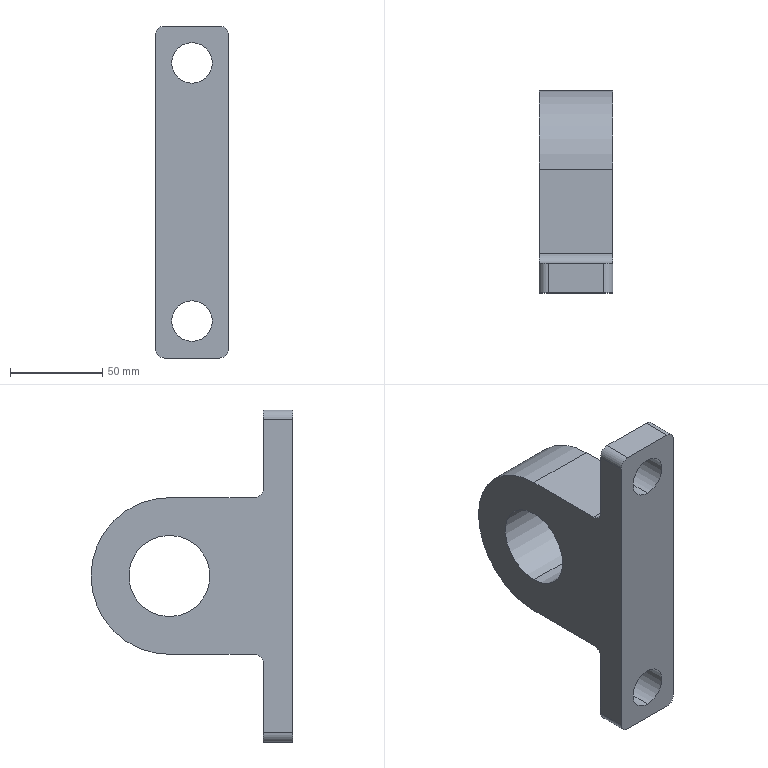Part | SolidWorks | features Extrusion 1, Fillet 1, ICE 1 | 1 solid | 22 faces | box 40 x 109.5 x 180 mm | volume 329190 mm3 | cylinder 13 | plane 9 | commonest cylinder face diameters 10 x6 22 x4 44 x2 85 x1
STEP:
#1=CARTESIAN_POINT('',(20.,67.,22.));
#2=VERTEX_POINT('',#1);
#3=CARTESIAN_POINT('',(20.,67.,-22.));
#4=VERTEX_POINT('',#3);
#5=CARTESIAN_POINT('',(20.,67.,0.));
#6=DIRECTION('',(1.,0.,0.));
#7=DIRECTION('',(0.,0.,-1.));
#8=AXIS2_PLACEMENT_3D('',#5,#6,#7);
#9=CIRCLE('',#8,22.);
#10=EDGE_CURVE('',#2,#4,#9,.T.);
#11=ORIENTED_EDGE('',*,*,#10,.T.);
#12=CARTESIAN_POINT('',(-20.,67.,-22.));
#13=VERTEX_POINT('',#12);
#14=CARTESIAN_POINT('',(20.,67.,-22.));
#15=DIRECTION('',(-1.,0.,0.));
#16=VECTOR('',#15,1000.);
#17=LINE('',#14,#16);
#18=EDGE_CURVE('',#4,#13,#17,.T.);
#19=ORIENTED_EDGE('',*,*,#18,.T.);
#20=CARTESIAN_POINT('',(-20.,67.,22.));
#21=VERTEX_POINT('',#20);
#22=CARTESIAN_POINT('',(-20.,67.,0.));
#23=DIRECTION('',(1.,0.,0.));
#24=DIRECTION('',(0.,0.,-1.));
#25=AXIS2_PLACEMENT_3D('',#22,#23,#24);
#26=CIRCLE('',#25,22.);
#27=EDGE_CURVE('',#21,#13,#26,.T.);
#28=ORIENTED_EDGE('',*,*,#27,.F.);
#29=CARTESIAN_POINT('',(20.,67.,22.));
#30=DIRECTION('',(-1.,0.,0.));
#31=VECTOR('',#30,1000.);
#32=LINE('',#29,#31);
#33=EDGE_CURVE('',#2,#21,#32,.T.);
#34=ORIENTED_EDGE('',*,*,#33,.F.);
#35=EDGE_LOOP('',(#11,#19,#28,#34));
#36=FACE_OUTER_BOUND('',#35,.T.);
#37=CARTESIAN_POINT('',(20.,67.,0.));
#38=DIRECTION('',(-1.,0.,0.));
#39=DIRECTION('',(0.,0.,1.));
#40=AXIS2_PLACEMENT_3D('',#37,#38,#39);
#41=CYLINDRICAL_SURFACE('',#40,22.);
#42=ADVANCED_FACE('',(#36),#41,.F.);
#43=CARTESIAN_POINT('',(0.,16.,59.));
#44=VERTEX_POINT('',#43);
#45=CARTESIAN_POINT('',(0.,16.,81.));
#46=VERTEX_POINT('',#45);
#47=CARTESIAN_POINT('',(0.,16.,70.));
#48=DIRECTION('',(0.,1.,0.));
#49=DIRECTION('',(0.,0.,-1.));
#50=AXIS2_PLACEMENT_3D('',#47,#48,#49);
#51=CIRCLE('',#50,11.);
#52=EDGE_CURVE('',#44,#46,#51,.T.);
#53=ORIENTED_EDGE('',*,*,#52,.T.);
#54=CARTESIAN_POINT('',(0.,0.,81.));
#55=VERTEX_POINT('',#54);
#56=CARTESIAN_POINT('',(0.,16.,81.));
#57=DIRECTION('',(0.,-1.,0.));
#58=VECTOR('',#57,1000.);
#59=LINE('',#56,#58);
#60=EDGE_CURVE('',#46,#55,#59,.T.);
#61=ORIENTED_EDGE('',*,*,#60,.T.);
#62=CARTESIAN_POINT('',(0.,0.,59.));
#63=VERTEX_POINT('',#62);
#64=CARTESIAN_POINT('',(0.,0.,70.));
#65=DIRECTION('',(0.,1.,0.));
#66=DIRECTION('',(0.,0.,-1.));
#67=AXIS2_PLACEMENT_3D('',#64,#65,#66);
#68=CIRCLE('',#67,11.);
#69=EDGE_CURVE('',#63,#55,#68,.T.);
#70=ORIENTED_EDGE('',*,*,#69,.F.);
#71=CARTESIAN_POINT('',(0.,16.,59.));
#72=DIRECTION('',(0.,-1.,0.));
#73=VECTOR('',#72,1000.);
#74=LINE('',#71,#73);
#75=EDGE_CURVE('',#44,#63,#74,.T.);
#76=ORIENTED_EDGE('',*,*,#75,.F.);
#77=EDGE_LOOP('',(#53,#61,#70,#76));
#78=FACE_OUTER_BOUND('',#77,.T.);
#79=CARTESIAN_POINT('',(0.,16.,70.));
#80=DIRECTION('',(0.,-1.,0.));
#81=DIRECTION('',(0.,0.,-1.));
#82=AXIS2_PLACEMENT_3D('',#79,#80,#81);
#83=CYLINDRICAL_SURFACE('',#82,11.);
#84=ADVANCED_FACE('',(#78),#83,.F.);
#85=CARTESIAN_POINT('',(0.,16.,-81.));
#86=VERTEX_POINT('',#85);
#87=CARTESIAN_POINT('',(0.,16.,-59.));
#88=VERTEX_POINT('',#87);
#89=CARTESIAN_POINT('',(0.,16.,-70.));
#90=DIRECTION('',(0.,1.,0.));
#91=DIRECTION('',(0.,0.,1.));
#92=AXIS2_PLACEMENT_3D('',#89,#90,#91);
#93=CIRCLE('',#92,11.);
#94=EDGE_CURVE('',#86,#88,#93,.T.);
#95=ORIENTED_EDGE('',*,*,#94,.T.);
#96=CARTESIAN_POINT('',(0.,0.,-59.));
#97=VERTEX_POINT('',#96);
#98=CARTESIAN_POINT('',(0.,16.,-59.));
#99=DIRECTION('',(0.,-1.,0.));
#100=VECTOR('',#99,1000.);
#101=LINE('',#98,#100);
#102=EDGE_CURVE('',#88,#97,#101,.T.);
#103=ORIENTED_EDGE('',*,*,#102,.T.);
#104=CARTESIAN_POINT('',(0.,0.,-81.));
#105=VERTEX_POINT('',#104);
#106=CARTESIAN_POINT('',(0.,0.,-70.));
#107=DIRECTION('',(0.,1.,0.));
#108=DIRECTION('',(0.,0.,1.));
#109=AXIS2_PLACEMENT_3D('',#106,#107,#108);
#110=CIRCLE('',#109,11.);
#111=EDGE_CURVE('',#105,#97,#110,.T.);
#112=ORIENTED_EDGE('',*,*,#111,.F.);
#113=CARTESIAN_POINT('',(0.,16.,-81.));
#114=DIRECTION('',(0.,-1.,0.));
#115=VECTOR('',#114,1000.);
#116=LINE('',#113,#115);
#117=EDGE_CURVE('',#86,#105,#116,.T.);
#118=ORIENTED_EDGE('',*,*,#117,.F.);
#119=EDGE_LOOP('',(#95,#103,#112,#118));
#120=FACE_OUTER_BOUND('',#119,.T.);
#121=CARTESIAN_POINT('',(0.,16.,-70.));
#122=DIRECTION('',(0.,-1.,0.));
#123=DIRECTION('',(0.,0.,-1.));
#124=AXIS2_PLACEMENT_3D('',#121,#122,#123);
#125=CYLINDRICAL_SURFACE('',#124,11.);
#126=ADVANCED_FACE('',(#120),#125,.F.);
#127=ORIENTED_EDGE('',*,*,#52,.F.);
#128=CARTESIAN_POINT('',(0.,16.,70.));
#129=DIRECTION('',(0.,1.,0.));
#130=DIRECTION('',(0.,0.,-1.));
#131=AXIS2_PLACEMENT_3D('',#128,#129,#130);
#132=CIRCLE('',#131,11.);
#133=EDGE_CURVE('',#46,#44,#132,.T.);
#134=ORIENTED_EDGE('',*,*,#133,.F.);
#135=EDGE_LOOP('',(#127,#134));
#136=FACE_BOUND('',#135,.T.);
#137=CARTESIAN_POINT('',(20.,16.,85.));
#138=VERTEX_POINT('',#137);
#139=CARTESIAN_POINT('',(20.,16.,47.5));
#140=VERTEX_POINT('',#139);
#141=CARTESIAN_POINT('',(20.,16.,-90.));
#142=DIRECTION('',(0.,0.,-1.));
#143=VECTOR('',#142,1000.);
#144=LINE('',#141,#143);
#145=EDGE_CURVE('',#138,#140,#144,.T.);
#146=ORIENTED_EDGE('',*,*,#145,.T.);
#147=CARTESIAN_POINT('',(-20.,16.,47.5));
#148=VERTEX_POINT('',#147);
#149=CARTESIAN_POINT('',(-20.,16.,47.5));
#150=DIRECTION('',(-1.,0.,0.));
#151=VECTOR('',#150,1000.);
#152=LINE('',#149,#151);
#153=EDGE_CURVE('',#140,#148,#152,.T.);
#154=ORIENTED_EDGE('',*,*,#153,.T.);
#155=CARTESIAN_POINT('',(-20.,16.,85.));
#156=VERTEX_POINT('',#155);
#157=CARTESIAN_POINT('',(-20.,16.,-90.));
#158=DIRECTION('',(0.,0.,1.));
#159=VECTOR('',#158,1000.);
#160=LINE('',#157,#159);
#161=EDGE_CURVE('',#148,#156,#160,.T.);
#162=ORIENTED_EDGE('',*,*,#161,.T.);
#163=CARTESIAN_POINT('',(-15.,16.,90.));
#164=VERTEX_POINT('',#163);
#165=CARTESIAN_POINT('',(-15.,16.,85.));
#166=DIRECTION('',(0.,1.,0.));
#167=DIRECTION('',(0.,0.,1.));
#168=AXIS2_PLACEMENT_3D('',#165,#166,#167);
#169=CIRCLE('',#168,5.);
#170=EDGE_CURVE('',#156,#164,#169,.T.);
#171=ORIENTED_EDGE('',*,*,#170,.T.);
#172=CARTESIAN_POINT('',(15.,16.,90.));
#173=VERTEX_POINT('',#172);
#174=CARTESIAN_POINT('',(-20.,16.,90.));
#175=DIRECTION('',(1.,0.,0.));
#176=VECTOR('',#175,1000.);
#177=LINE('',#174,#176);
#178=EDGE_CURVE('',#164,#173,#177,.T.);
#179=ORIENTED_EDGE('',*,*,#178,.T.);
#180=CARTESIAN_POINT('',(15.,16.,85.));
#181=DIRECTION('',(0.,1.,0.));
#182=DIRECTION('',(0.,0.,1.));
#183=AXIS2_PLACEMENT_3D('',#180,#181,#182);
#184=CIRCLE('',#183,5.);
#185=EDGE_CURVE('',#173,#138,#184,.T.);
#186=ORIENTED_EDGE('',*,*,#185,.T.);
#187=EDGE_LOOP('',(#146,#154,#162,#171,#179,#186));
#188=FACE_OUTER_BOUND('',#187,.T.);
#189=CARTESIAN_POINT('',(-20.,16.,90.));
#190=DIRECTION('',(0.,1.,0.));
#191=DIRECTION('',(0.,0.,1.));
#192=AXIS2_PLACEMENT_3D('',#189,#190,#191);
#193=PLANE('',#192);
#194=ADVANCED_FACE('',(#136,#188),#193,.T.);
#195=CARTESIAN_POINT('',(20.,16.,-47.5));
#196=VERTEX_POINT('',#195);
#197=CARTESIAN_POINT('',(20.,16.,-85.));
#198=VERTEX_POINT('',#197);
#199=CARTESIAN_POINT('',(20.,16.,-90.));
#200=DIRECTION('',(0.,0.,-1.));
#201=VECTOR('',#200,1000.);
#202=LINE('',#199,#201);
#203=EDGE_CURVE('',#196,#198,#202,.T.);
#204=ORIENTED_EDGE('',*,*,#203,.T.);
#205=CARTESIAN_POINT('',(15.,16.,-90.));
#206=VERTEX_POINT('',#205);
#207=CARTESIAN_POINT('',(15.,16.,-85.));
#208=DIRECTION('',(0.,1.,0.));
#209=DIRECTION('',(0.,0.,1.));
#210=AXIS2_PLACEMENT_3D('',#207,#208,#209);
#211=CIRCLE('',#210,5.);
#212=EDGE_CURVE('',#198,#206,#211,.T.);
#213=ORIENTED_EDGE('',*,*,#212,.T.);
#214=CARTESIAN_POINT('',(-15.,16.,-90.));
#215=VERTEX_POINT('',#214);
#216=CARTESIAN_POINT('',(-20.,16.,-90.));
#217=DIRECTION('',(-1.,0.,0.));
#218=VECTOR('',#217,1000.);
#219=LINE('',#216,#218);
#220=EDGE_CURVE('',#206,#215,#219,.T.);
#221=ORIENTED_EDGE('',*,*,#220,.T.);
#222=CARTESIAN_POINT('',(-20.,16.,-85.));
#223=VERTEX_POINT('',#222);
#224=CARTESIAN_POINT('',(-15.,16.,-85.));
#225=DIRECTION('',(0.,1.,0.));
#226=DIRECTION('',(0.,0.,1.));
#227=AXIS2_PLACEMENT_3D('',#224,#225,#226);
#228=CIRCLE('',#227,5.);
#229=EDGE_CURVE('',#215,#223,#228,.T.);
#230=ORIENTED_EDGE('',*,*,#229,.T.);
#231=CARTESIAN_POINT('',(-20.,16.,-47.5));
#232=VERTEX_POINT('',#231);
#233=CARTESIAN_POINT('',(-20.,16.,-90.));
#234=DIRECTION('',(0.,0.,1.));
#235=VECTOR('',#234,1000.);
#236=LINE('',#233,#235);
#237=EDGE_CURVE('',#223,#232,#236,.T.);
#238=ORIENTED_EDGE('',*,*,#237,.T.);
#239=CARTESIAN_POINT('',(-20.,16.,-47.5));
#240=DIRECTION('',(1.,0.,0.));
#241=VECTOR('',#240,1000.);
#242=LINE('',#239,#241);
#243=EDGE_CURVE('',#232,#196,#242,.T.);
#244=ORIENTED_EDGE('',*,*,#243,.T.);
#245=EDGE_LOOP('',(#204,#213,#221,#230,#238,#244));
#246=FACE_OUTER_BOUND('',#245,.T.);
#247=ORIENTED_EDGE('',*,*,#94,.F.);
#248=CARTESIAN_POINT('',(0.,16.,-70.));
#249=DIRECTION('',(0.,1.,0.));
#250=DIRECTION('',(0.,0.,1.));
#251=AXIS2_PLACEMENT_3D('',#248,#249,#250);
#252=CIRCLE('',#251,11.);
#253=EDGE_CURVE('',#88,#86,#252,.T.);
#254=ORIENTED_EDGE('',*,*,#253,.F.);
#255=EDGE_LOOP('',(#247,#254));
#256=FACE_BOUND('',#255,.T.);
#257=CARTESIAN_POINT('',(-20.,16.,90.));
#258=DIRECTION('',(0.,1.,0.));
#259=DIRECTION('',(0.,0.,1.));
#260=AXIS2_PLACEMENT_3D('',#257,#258,#259);
#261=PLANE('',#260);
#262=ADVANCED_FACE('',(#246,#256),#261,.T.);
#263=ORIENTED_EDGE('',*,*,#111,.T.);
#264=CARTESIAN_POINT('',(0.,0.,-70.));
#265=DIRECTION('',(0.,1.,0.));
#266=DIRECTION('',(0.,0.,1.));
#267=AXIS2_PLACEMENT_3D('',#264,#265,#266);
#268=CIRCLE('',#267,11.);
#269=EDGE_CURVE('',#97,#105,#268,.T.);
#270=ORIENTED_EDGE('',*,*,#269,.T.);
#271=EDGE_LOOP('',(#263,#270));
#272=FACE_BOUND('',#271,.T.);
#273=CARTESIAN_POINT('',(20.,0.,85.));
#274=VERTEX_POINT('',#273);
#275=CARTESIAN_POINT('',(20.,0.,-85.));
#276=VERTEX_POINT('',#275);
#277=CARTESIAN_POINT('',(20.,0.,-90.));
#278=DIRECTION('',(0.,0.,-1.));
#279=VECTOR('',#278,1000.);
#280=LINE('',#277,#279);
#281=EDGE_CURVE('',#274,#276,#280,.T.);
#282=ORIENTED_EDGE('',*,*,#281,.F.);
#283=CARTESIAN_POINT('',(15.,0.,90.));
#284=VERTEX_POINT('',#283);
#285=CARTESIAN_POINT('',(15.,0.,85.));
#286=DIRECTION('',(0.,-1.,0.));
#287=DIRECTION('',(0.,0.,1.));
#288=AXIS2_PLACEMENT_3D('',#285,#286,#287);
#289=CIRCLE('',#288,5.);
#290=EDGE_CURVE('',#274,#284,#289,.T.);
#291=ORIENTED_EDGE('',*,*,#290,.T.);
#292=CARTESIAN_POINT('',(-15.,0.,90.));
#293=VERTEX_POINT('',#292);
#294=CARTESIAN_POINT('',(-20.,0.,90.));
#295=DIRECTION('',(1.,0.,0.));
#296=VECTOR('',#295,1000.);
#297=LINE('',#294,#296);
#298=EDGE_CURVE('',#293,#284,#297,.T.);
#299=ORIENTED_EDGE('',*,*,#298,.F.);
#300=CARTESIAN_POINT('',(-20.,0.,85.));
#301=VERTEX_POINT('',#300);
#302=CARTESIAN_POINT('',(-15.,0.,85.));
#303=DIRECTION('',(0.,-1.,0.));
#304=DIRECTION('',(0.,0.,1.));
#305=AXIS2_PLACEMENT_3D('',#302,#303,#304);
#306=CIRCLE('',#305,5.);
#307=EDGE_CURVE('',#293,#301,#306,.T.);
#308=ORIENTED_EDGE('',*,*,#307,.T.);
#309=CARTESIAN_POINT('',(-20.,0.,-85.));
#310=VERTEX_POINT('',#309);
#311=CARTESIAN_POINT('',(-20.,0.,-90.));
#312=DIRECTION('',(0.,0.,1.));
#313=VECTOR('',#312,1000.);
#314=LINE('',#311,#313);
#315=EDGE_CURVE('',#310,#301,#314,.T.);
#316=ORIENTED_EDGE('',*,*,#315,.F.);
#317=CARTESIAN_POINT('',(-15.,0.,-90.));
#318=VERTEX_POINT('',#317);
#319=CARTESIAN_POINT('',(-15.,0.,-85.));
#320=DIRECTION('',(0.,-1.,0.));
#321=DIRECTION('',(0.,0.,1.));
#322=AXIS2_PLACEMENT_3D('',#319,#320,#321);
#323=CIRCLE('',#322,5.);
#324=EDGE_CURVE('',#310,#318,#323,.T.);
#325=ORIENTED_EDGE('',*,*,#324,.T.);
#326=CARTESIAN_POINT('',(15.,0.,-90.));
#327=VERTEX_POINT('',#326);
#328=CARTESIAN_POINT('',(-20.,0.,-90.));
#329=DIRECTION('',(-1.,0.,0.));
#330=VECTOR('',#329,1000.);
#331=LINE('',#328,#330);
#332=EDGE_CURVE('',#327,#318,#331,.T.);
#333=ORIENTED_EDGE('',*,*,#332,.F.);
#334=CARTESIAN_POINT('',(15.,0.,-85.));
#335=DIRECTION('',(0.,-1.,0.));
#336=DIRECTION('',(0.,0.,1.));
#337=AXIS2_PLACEMENT_3D('',#334,#335,#336);
#338=CIRCLE('',#337,5.);
#339=EDGE_CURVE('',#327,#276,#338,.T.);
#340=ORIENTED_EDGE('',*,*,#339,.T.);
#341=EDGE_LOOP('',(#282,#291,#299,#308,#316,#325,#333,#340));
#342=FACE_OUTER_BOUND('',#341,.T.);
#343=ORIENTED_EDGE('',*,*,#69,.T.);
#344=CARTESIAN_POINT('',(0.,0.,70.));
#345=DIRECTION('',(0.,1.,0.));
#346=DIRECTION('',(0.,0.,-1.));
#347=AXIS2_PLACEMENT_3D('',#344,#345,#346);
#348=CIRCLE('',#347,11.);
#349=EDGE_CURVE('',#55,#63,#348,.T.);
#350=ORIENTED_EDGE('',*,*,#349,.T.);
#351=EDGE_LOOP('',(#343,#350));
#352=FACE_BOUND('',#351,.T.);
#353=CARTESIAN_POINT('',(-20.,0.,90.));
#354=DIRECTION('',(0.,1.,0.));
#355=DIRECTION('',(0.,0.,1.));
#356=AXIS2_PLACEMENT_3D('',#353,#354,#355);
#357=PLANE('',#356);
#358=ADVANCED_FACE('',(#272,#342,#352),#357,.F.);
#359=ORIENTED_EDGE('',*,*,#315,.T.);
#360=CARTESIAN_POINT('',(-20.,16.,85.));
#361=DIRECTION('',(0.,1.,0.));
#362=VECTOR('',#361,1000.);
#363=LINE('',#360,#362);
#364=EDGE_CURVE('',#301,#156,#363,.T.);
#365=ORIENTED_EDGE('',*,*,#364,.T.);
#366=ORIENTED_EDGE('',*,*,#161,.F.);
#367=CARTESIAN_POINT('',(-20.,21.,42.5));
#368=VERTEX_POINT('',#367);
#369=CARTESIAN_POINT('',(-20.,21.,47.5));
#370=DIRECTION('',(1.,0.,0.));
#371=DIRECTION('',(0.,0.,-1.));
#372=AXIS2_PLACEMENT_3D('',#369,#370,#371);
#373=CIRCLE('',#372,5.);
#374=EDGE_CURVE('',#148,#368,#373,.T.);
#375=ORIENTED_EDGE('',*,*,#374,.T.);
#376=CARTESIAN_POINT('',(-20.,67.,42.5));
#377=VERTEX_POINT('',#376);
#378=CARTESIAN_POINT('',(-20.,67.,42.5));
#379=DIRECTION('',(0.,-1.,0.));
#380=VECTOR('',#379,1000.);
#381=LINE('',#378,#380);
#382=EDGE_CURVE('',#377,#368,#381,.T.);
#383=ORIENTED_EDGE('',*,*,#382,.F.);
#384=CARTESIAN_POINT('',(-20.,67.,-42.5));
#385=VERTEX_POINT('',#384);
#386=CARTESIAN_POINT('',(-20.,67.,0.));
#387=DIRECTION('',(1.,0.,0.));
#388=DIRECTION('',(0.,0.,-1.));
#389=AXIS2_PLACEMENT_3D('',#386,#387,#388);
#390=CIRCLE('',#389,42.5);
#391=EDGE_CURVE('',#385,#377,#390,.T.);
#392=ORIENTED_EDGE('',*,*,#391,.F.);
#393=CARTESIAN_POINT('',(-20.,21.,-42.5));
#394=VERTEX_POINT('',#393);
#395=CARTESIAN_POINT('',(-20.,67.,-42.5));
#396=DIRECTION('',(0.,1.,0.));
#397=VECTOR('',#396,1000.);
#398=LINE('',#395,#397);
#399=EDGE_CURVE('',#394,#385,#398,.T.);
#400=ORIENTED_EDGE('',*,*,#399,.F.);
#401=CARTESIAN_POINT('',(-20.,21.,-47.5));
#402=DIRECTION('',(1.,0.,0.));
#403=DIRECTION('',(0.,0.,-1.));
#404=AXIS2_PLACEMENT_3D('',#401,#402,#403);
#405=CIRCLE('',#404,5.);
#406=EDGE_CURVE('',#394,#232,#405,.T.);
#407=ORIENTED_EDGE('',*,*,#406,.T.);
#408=ORIENTED_EDGE('',*,*,#237,.F.);
#409=CARTESIAN_POINT('',(-20.,16.,-85.));
#410=DIRECTION('',(0.,-1.,0.));
#411=VECTOR('',#410,1000.);
#412=LINE('',#409,#411);
#413=EDGE_CURVE('',#223,#310,#412,.T.);
#414=ORIENTED_EDGE('',*,*,#413,.T.);
#415=EDGE_LOOP('',(#359,#365,#366,#375,#383,#392,#400,#407,#408,#414));
#416=FACE_OUTER_BOUND('',#415,.T.);
#417=ORIENTED_EDGE('',*,*,#27,.T.);
#418=CARTESIAN_POINT('',(-20.,67.,0.));
#419=DIRECTION('',(1.,0.,0.));
#420=DIRECTION('',(0.,0.,-1.));
#421=AXIS2_PLACEMENT_3D('',#418,#419,#420);
#422=CIRCLE('',#421,22.);
#423=EDGE_CURVE('',#13,#21,#422,.T.);
#424=ORIENTED_EDGE('',*,*,#423,.T.);
#425=EDGE_LOOP('',(#417,#424));
#426=FACE_BOUND('',#425,.T.);
#427=CARTESIAN_POINT('',(-20.,16.,-90.));
#428=DIRECTION('',(1.,0.,0.));
#429=DIRECTION('',(0.,0.,-1.));
#430=AXIS2_PLACEMENT_3D('',#427,#428,#429);
#431=PLANE('',#430);
#432=ADVANCED_FACE('',(#416,#426),#431,.F.);
#433=ORIENTED_EDGE('',*,*,#298,.T.);
#434=CARTESIAN_POINT('',(15.,16.,90.));
#435=DIRECTION('',(0.,1.,0.));
#436=VECTOR('',#435,1000.);
#437=LINE('',#434,#436);
#438=EDGE_CURVE('',#284,#173,#437,.T.);
#439=ORIENTED_EDGE('',*,*,#438,.T.);
#440=ORIENTED_EDGE('',*,*,#178,.F.);
#441=CARTESIAN_POINT('',(-15.,16.,90.));
#442=DIRECTION('',(0.,-1.,0.));
#443=VECTOR('',#442,1000.);
#444=LINE('',#441,#443);
#445=EDGE_CURVE('',#164,#293,#444,.T.);
#446=ORIENTED_EDGE('',*,*,#445,.T.);
#447=EDGE_LOOP('',(#433,#439,#440,#446));
#448=FACE_OUTER_BOUND('',#447,.T.);
#449=CARTESIAN_POINT('',(-20.,16.,90.));
#450=DIRECTION('',(0.,0.,-1.));
#451=DIRECTION('',(-1.,0.,0.));
#452=AXIS2_PLACEMENT_3D('',#449,#450,#451);
#453=PLANE('',#452);
#454=ADVANCED_FACE('',(#448),#453,.F.);
#455=ORIENTED_EDGE('',*,*,#145,.F.);
#456=CARTESIAN_POINT('',(20.,16.,85.));
#457=DIRECTION('',(0.,-1.,0.));
#458=VECTOR('',#457,1000.);
#459=LINE('',#456,#458);
#460=EDGE_CURVE('',#138,#274,#459,.T.);
#461=ORIENTED_EDGE('',*,*,#460,.T.);
#462=ORIENTED_EDGE('',*,*,#281,.T.);
#463=CARTESIAN_POINT('',(20.,16.,-85.));
#464=DIRECTION('',(0.,1.,0.));
#465=VECTOR('',#464,1000.);
#466=LINE('',#463,#465);
#467=EDGE_CURVE('',#276,#198,#466,.T.);
#468=ORIENTED_EDGE('',*,*,#467,.T.);
#469=ORIENTED_EDGE('',*,*,#203,.F.);
#470=CARTESIAN_POINT('',(20.,21.,-42.5));
#471=VERTEX_POINT('',#470);
#472=CARTESIAN_POINT('',(20.,21.,-47.5));
#473=DIRECTION('',(-1.,0.,0.));
#474=DIRECTION('',(0.,0.,1.));
#475=AXIS2_PLACEMENT_3D('',#472,#473,#474);
#476=CIRCLE('',#475,5.);
#477=EDGE_CURVE('',#196,#471,#476,.T.);
#478=ORIENTED_EDGE('',*,*,#477,.T.);
#479=CARTESIAN_POINT('',(20.,67.,-42.5));
#480=VERTEX_POINT('',#479);
#481=CARTESIAN_POINT('',(20.,67.,-42.5));
#482=DIRECTION('',(0.,1.,0.));
#483=VECTOR('',#482,1000.);
#484=LINE('',#481,#483);
#485=EDGE_CURVE('',#471,#480,#484,.T.);
#486=ORIENTED_EDGE('',*,*,#485,.T.);
#487=CARTESIAN_POINT('',(20.,67.,42.5));
#488=VERTEX_POINT('',#487);
#489=CARTESIAN_POINT('',(20.,67.,0.));
#490=DIRECTION('',(1.,0.,0.));
#491=DIRECTION('',(0.,0.,-1.));
#492=AXIS2_PLACEMENT_3D('',#489,#490,#491);
#493=CIRCLE('',#492,42.5);
#494=EDGE_CURVE('',#480,#488,#493,.T.);
#495=ORIENTED_EDGE('',*,*,#494,.T.);
#496=CARTESIAN_POINT('',(20.,21.,42.5));
#497=VERTEX_POINT('',#496);
#498=CARTESIAN_POINT('',(20.,67.,42.5));
#499=DIRECTION('',(0.,-1.,0.));
#500=VECTOR('',#499,1000.);
#501=LINE('',#498,#500);
#502=EDGE_CURVE('',#488,#497,#501,.T.);
#503=ORIENTED_EDGE('',*,*,#502,.T.);
#504=CARTESIAN_POINT('',(20.,21.,47.5));
#505=DIRECTION('',(-1.,0.,0.));
#506=DIRECTION('',(0.,0.,1.));
#507=AXIS2_PLACEMENT_3D('',#504,#505,#506);
#508=CIRCLE('',#507,5.);
#509=EDGE_CURVE('',#497,#140,#508,.T.);
#510=ORIENTED_EDGE('',*,*,#509,.T.);
#511=EDGE_LOOP('',(#455,#461,#462,#468,#469,#478,#486,#495,#503,#510));
#512=FACE_OUTER_BOUND('',#511,.T.);
#513=ORIENTED_EDGE('',*,*,#10,.F.);
#514=CARTESIAN_POINT('',(20.,67.,0.));
#515=DIRECTION('',(1.,0.,0.));
#516=DIRECTION('',(0.,0.,-1.));
#517=AXIS2_PLACEMENT_3D('',#514,#515,#516);
#518=CIRCLE('',#517,22.);
#519=EDGE_CURVE('',#4,#2,#518,.T.);
#520=ORIENTED_EDGE('',*,*,#519,.F.);
#521=EDGE_LOOP('',(#513,#520));
#522=FACE_BOUND('',#521,.T.);
#523=CARTESIAN_POINT('',(20.,16.,-90.));
#524=DIRECTION('',(-1.,0.,0.));
#525=DIRECTION('',(0.,0.,1.));
#526=AXIS2_PLACEMENT_3D('',#523,#524,#525);
#527=PLANE('',#526);
#528=ADVANCED_FACE('',(#512,#522),#527,.F.);
#529=ORIENTED_EDGE('',*,*,#220,.F.);
#530=CARTESIAN_POINT('',(15.,16.,-90.));
#531=DIRECTION('',(0.,-1.,0.));
#532=VECTOR('',#531,1000.);
#533=LINE('',#530,#532);
#534=EDGE_CURVE('',#206,#327,#533,.T.);
#535=ORIENTED_EDGE('',*,*,#534,.T.);
#536=ORIENTED_EDGE('',*,*,#332,.T.);
#537=CARTESIAN_POINT('',(-15.,16.,-90.));
#538=DIRECTION('',(0.,1.,0.));
#539=VECTOR('',#538,1000.);
#540=LINE('',#537,#539);
#541=EDGE_CURVE('',#318,#215,#540,.T.);
#542=ORIENTED_EDGE('',*,*,#541,.T.);
#543=EDGE_LOOP('',(#529,#535,#536,#542));
#544=FACE_OUTER_BOUND('',#543,.T.);
#545=CARTESIAN_POINT('',(-20.,16.,-90.));
#546=DIRECTION('',(0.,0.,1.));
#547=DIRECTION('',(1.,0.,0.));
#548=AXIS2_PLACEMENT_3D('',#545,#546,#547);
#549=PLANE('',#548);
#550=ADVANCED_FACE('',(#544),#549,.F.);
#551=ORIENTED_EDGE('',*,*,#102,.F.);
#552=ORIENTED_EDGE('',*,*,#253,.T.);
#553=ORIENTED_EDGE('',*,*,#117,.T.);
#554=ORIENTED_EDGE('',*,*,#269,.F.);
#555=EDGE_LOOP('',(#551,#552,#553,#554));
#556=FACE_OUTER_BOUND('',#555,.T.);
#557=CARTESIAN_POINT('',(0.,16.,-70.));
#558=DIRECTION('',(0.,-1.,0.));
#559=DIRECTION('',(0.,0.,-1.));
#560=AXIS2_PLACEMENT_3D('',#557,#558,#559);
#561=CYLINDRICAL_SURFACE('',#560,11.);
#562=ADVANCED_FACE('',(#556),#561,.F.);
#563=ORIENTED_EDGE('',*,*,#60,.F.);
#564=ORIENTED_EDGE('',*,*,#133,.T.);
#565=ORIENTED_EDGE('',*,*,#75,.T.);
#566=ORIENTED_EDGE('',*,*,#349,.F.);
#567=EDGE_LOOP('',(#563,#564,#565,#566));
#568=FACE_OUTER_BOUND('',#567,.T.);
#569=CARTESIAN_POINT('',(0.,16.,70.));
#570=DIRECTION('',(0.,-1.,0.));
#571=DIRECTION('',(0.,0.,-1.));
#572=AXIS2_PLACEMENT_3D('',#569,#570,#571);
#573=CYLINDRICAL_SURFACE('',#572,11.);
#574=ADVANCED_FACE('',(#568),#573,.F.);
#575=ORIENTED_EDGE('',*,*,#391,.T.);
#576=CARTESIAN_POINT('',(20.,67.,42.5));
#577=DIRECTION('',(-1.,0.,0.));
#578=VECTOR('',#577,1000.);
#579=LINE('',#576,#578);
#580=EDGE_CURVE('',#488,#377,#579,.T.);
#581=ORIENTED_EDGE('',*,*,#580,.F.);
#582=ORIENTED_EDGE('',*,*,#494,.F.);
#583=CARTESIAN_POINT('',(20.,67.,-42.5));
#584=DIRECTION('',(-1.,0.,0.));
#585=VECTOR('',#584,1000.);
#586=LINE('',#583,#585);
#587=EDGE_CURVE('',#480,#385,#586,.T.);
#588=ORIENTED_EDGE('',*,*,#587,.T.);
#589=EDGE_LOOP('',(#575,#581,#582,#588));
#590=FACE_OUTER_BOUND('',#589,.T.);
#591=CARTESIAN_POINT('',(20.,67.,0.));
#592=DIRECTION('',(-1.,0.,0.));
#593=DIRECTION('',(0.,0.,1.));
#594=AXIS2_PLACEMENT_3D('',#591,#592,#593);
#595=CYLINDRICAL_SURFACE('',#594,42.5);
#596=ADVANCED_FACE('',(#590),#595,.T.);
#597=ORIENTED_EDGE('',*,*,#382,.T.);
#598=CARTESIAN_POINT('',(20.,21.,42.5));
#599=DIRECTION('',(1.,0.,0.));
#600=VECTOR('',#599,1000.);
#601=LINE('',#598,#600);
#602=EDGE_CURVE('',#368,#497,#601,.T.);
#603=ORIENTED_EDGE('',*,*,#602,.T.);
#604=ORIENTED_EDGE('',*,*,#502,.F.);
#605=ORIENTED_EDGE('',*,*,#580,.T.);
#606=EDGE_LOOP('',(#597,#603,#604,#605));
#607=FACE_OUTER_BOUND('',#606,.T.);
#608=CARTESIAN_POINT('',(20.,67.,42.5));
#609=DIRECTION('',(0.,0.,-1.));
#610=DIRECTION('',(0.,1.,0.));
#611=AXIS2_PLACEMENT_3D('',#608,#609,#610);
#612=PLANE('',#611);
#613=ADVANCED_FACE('',(#607),#612,.F.);
#614=ORIENTED_EDGE('',*,*,#485,.F.);
#615=CARTESIAN_POINT('',(20.,21.,-42.5));
#616=DIRECTION('',(-1.,0.,0.));
#617=VECTOR('',#616,1000.);
#618=LINE('',#615,#617);
#619=EDGE_CURVE('',#471,#394,#618,.T.);
#620=ORIENTED_EDGE('',*,*,#619,.T.);
#621=ORIENTED_EDGE('',*,*,#399,.T.);
#622=ORIENTED_EDGE('',*,*,#587,.F.);
#623=EDGE_LOOP('',(#614,#620,#621,#622));
#624=FACE_OUTER_BOUND('',#623,.T.);
#625=CARTESIAN_POINT('',(20.,67.,-42.5));
#626=DIRECTION('',(0.,0.,1.));
#627=DIRECTION('',(0.,-1.,0.));
#628=AXIS2_PLACEMENT_3D('',#625,#626,#627);
#629=PLANE('',#628);
#630=ADVANCED_FACE('',(#624),#629,.F.);
#631=ORIENTED_EDGE('',*,*,#18,.F.);
#632=ORIENTED_EDGE('',*,*,#519,.T.);
#633=ORIENTED_EDGE('',*,*,#33,.T.);
#634=ORIENTED_EDGE('',*,*,#423,.F.);
#635=EDGE_LOOP('',(#631,#632,#633,#634));
#636=FACE_OUTER_BOUND('',#635,.T.);
#637=CARTESIAN_POINT('',(20.,67.,0.));
#638=DIRECTION('',(-1.,0.,0.));
#639=DIRECTION('',(0.,0.,1.));
#640=AXIS2_PLACEMENT_3D('',#637,#638,#639);
#641=CYLINDRICAL_SURFACE('',#640,22.);
#642=ADVANCED_FACE('',(#636),#641,.F.);
#643=ORIENTED_EDGE('',*,*,#509,.F.);
#644=ORIENTED_EDGE('',*,*,#602,.F.);
#645=ORIENTED_EDGE('',*,*,#374,.F.);
#646=ORIENTED_EDGE('',*,*,#153,.F.);
#647=EDGE_LOOP('',(#643,#644,#645,#646));
#648=FACE_OUTER_BOUND('',#647,.T.);
#649=CARTESIAN_POINT('',(-20.,21.,47.5));
#650=DIRECTION('',(-1.,0.,0.));
#651=DIRECTION('',(0.,0.,1.));
#652=AXIS2_PLACEMENT_3D('',#649,#650,#651);
#653=CYLINDRICAL_SURFACE('',#652,5.);
#654=ADVANCED_FACE('',(#648),#653,.F.);
#655=ORIENTED_EDGE('',*,*,#185,.F.);
#656=ORIENTED_EDGE('',*,*,#438,.F.);
#657=ORIENTED_EDGE('',*,*,#290,.F.);
#658=ORIENTED_EDGE('',*,*,#460,.F.);
#659=EDGE_LOOP('',(#655,#656,#657,#658));
#660=FACE_OUTER_BOUND('',#659,.T.);
#661=CARTESIAN_POINT('',(15.,16.,85.));
#662=DIRECTION('',(0.,-1.,0.));
#663=DIRECTION('',(0.,0.,-1.));
#664=AXIS2_PLACEMENT_3D('',#661,#662,#663);
#665=CYLINDRICAL_SURFACE('',#664,5.);
#666=ADVANCED_FACE('',(#660),#665,.T.);
#667=ORIENTED_EDGE('',*,*,#170,.F.);
#668=ORIENTED_EDGE('',*,*,#364,.F.);
#669=ORIENTED_EDGE('',*,*,#307,.F.);
#670=ORIENTED_EDGE('',*,*,#445,.F.);
#671=EDGE_LOOP('',(#667,#668,#669,#670));
#672=FACE_OUTER_BOUND('',#671,.T.);
#673=CARTESIAN_POINT('',(-15.,16.,85.));
#674=DIRECTION('',(0.,-1.,0.));
#675=DIRECTION('',(0.,0.,-1.));
#676=AXIS2_PLACEMENT_3D('',#673,#674,#675);
#677=CYLINDRICAL_SURFACE('',#676,5.);
#678=ADVANCED_FACE('',(#672),#677,.T.);
#679=ORIENTED_EDGE('',*,*,#212,.F.);
#680=ORIENTED_EDGE('',*,*,#467,.F.);
#681=ORIENTED_EDGE('',*,*,#339,.F.);
#682=ORIENTED_EDGE('',*,*,#534,.F.);
#683=EDGE_LOOP('',(#679,#680,#681,#682));
#684=FACE_OUTER_BOUND('',#683,.T.);
#685=CARTESIAN_POINT('',(15.,16.,-85.));
#686=DIRECTION('',(0.,-1.,0.));
#687=DIRECTION('',(0.,0.,-1.));
#688=AXIS2_PLACEMENT_3D('',#685,#686,#687);
#689=CYLINDRICAL_SURFACE('',#688,5.);
#690=ADVANCED_FACE('',(#684),#689,.T.);
#691=ORIENTED_EDGE('',*,*,#229,.F.);
#692=ORIENTED_EDGE('',*,*,#541,.F.);
#693=ORIENTED_EDGE('',*,*,#324,.F.);
#694=ORIENTED_EDGE('',*,*,#413,.F.);
#695=EDGE_LOOP('',(#691,#692,#693,#694));
#696=FACE_OUTER_BOUND('',#695,.T.);
#697=CARTESIAN_POINT('',(-15.,16.,-85.));
#698=DIRECTION('',(0.,-1.,0.));
#699=DIRECTION('',(0.,0.,-1.));
#700=AXIS2_PLACEMENT_3D('',#697,#698,#699);
#701=CYLINDRICAL_SURFACE('',#700,5.);
#702=ADVANCED_FACE('',(#696),#701,.T.);
#703=ORIENTED_EDGE('',*,*,#477,.F.);
#704=ORIENTED_EDGE('',*,*,#243,.F.);
#705=ORIENTED_EDGE('',*,*,#406,.F.);
#706=ORIENTED_EDGE('',*,*,#619,.F.);
#707=EDGE_LOOP('',(#703,#704,#705,#706));
#708=FACE_OUTER_BOUND('',#707,.T.);
#709=CARTESIAN_POINT('',(20.,21.,-47.5));
#710=DIRECTION('',(-1.,0.,0.));
#711=DIRECTION('',(0.,0.,1.));
#712=AXIS2_PLACEMENT_3D('',#709,#710,#711);
#713=CYLINDRICAL_SURFACE('',#712,5.);
#714=ADVANCED_FACE('',(#708),#713,.F.);
#715=CLOSED_SHELL('',(#42,#84,#126,#194,#262,#358,#432,#454,#528,#550,#562,#574,#596,#613,#630,#642,#654,#666,#678,#690,#702,#714));
#716=MANIFOLD_SOLID_BREP('',#715);
#717=CARTESIAN_POINT('',(0.,0.,0.));
#718=DIRECTION('',(0.,0.,1.));
#719=DIRECTION('',(1.,0.,0.));
#720=AXIS2_PLACEMENT_3D('',#717,#718,#719);
#721=(LENGTH_UNIT()NAMED_UNIT(*)SI_UNIT(.MILLI.,.METRE.));
#722=UNCERTAINTY_MEASURE_WITH_UNIT(LENGTH_MEASURE(0.00001),#721,'','');
#723=(NAMED_UNIT(*)PLANE_ANGLE_UNIT()SI_UNIT($,.RADIAN.));
#724=(NAMED_UNIT(*)SI_UNIT($,.STERADIAN.)SOLID_ANGLE_UNIT());
#725=(GEOMETRIC_REPRESENTATION_CONTEXT(3)GLOBAL_UNCERTAINTY_ASSIGNED_CONTEXT((#722))GLOBAL_UNIT_ASSIGNED_CONTEXT((#721,#723,#724))REPRESENTATION_CONTEXT('',''));
#726=ADVANCED_BREP_SHAPE_REPRESENTATION('',(#716,#720),#725);